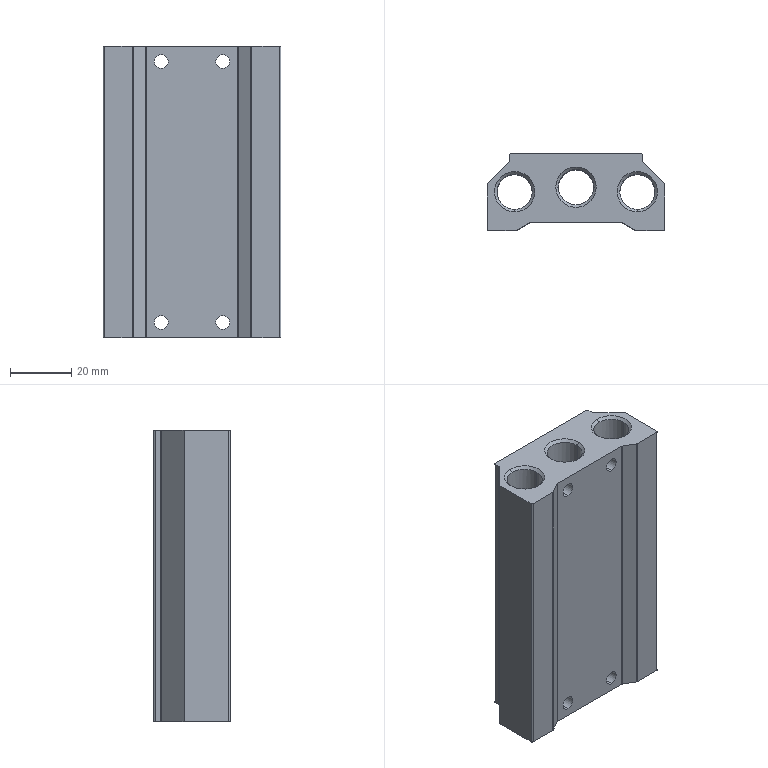Part | STEP file | 100M-4F | 1 solid | 130 faces | box 58 x 25 x 95 mm | volume 84414 mm3 | cylinder 64 | cone 44 | plane 22 | commonest cylinder face diameters 8 x24 2.459 x16 1 x10 4.5 x8 11.445 x6